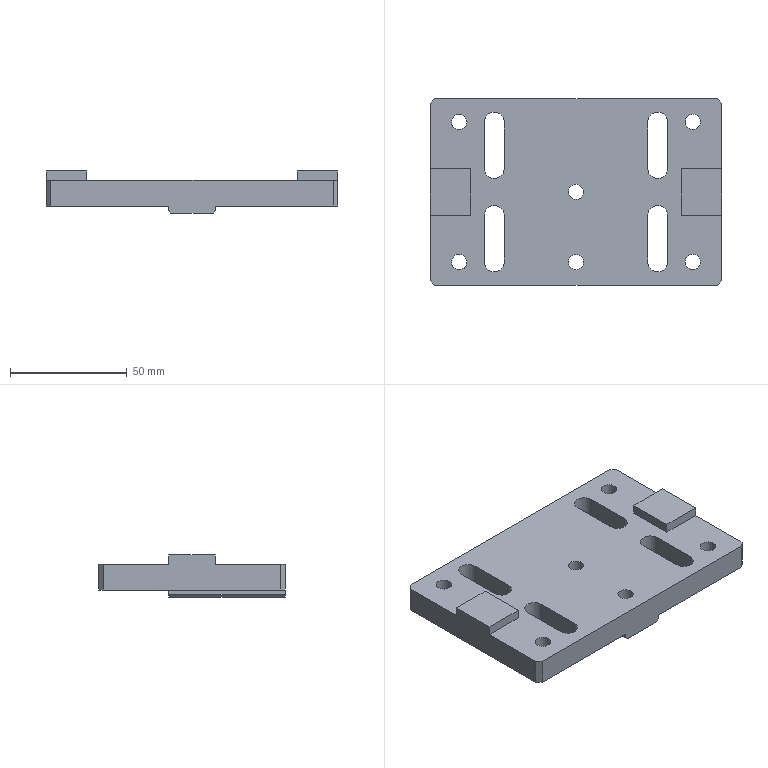NC program | NX | posted with a generic post | part box 125 x 80 x 18 mm
Lines 1 to 631 of 3483:
N10 G17 G21 G94 G90
(FLOOR_WALL , TOOL : D63)
N12 T01 M6
N14 G54
N16 G17 G0 G90 X97. Y-39.997 S6500 M3
N18 G43 Z30. H1
N20 Z3.
N22 G94 G1 Z0. F1500.
N24 X94.
N26 X-94.
N28 Y-32.029
N30 Y-12.599
N32 X94.
N34 Y14.8
N36 X-94.
N38 X-97.
N40 Z3.
N42 G0 Z30.
N44 M5
(FLOOR_WALL_1 , TOOL : D10)
N46 T04 M6
N48 G54
N50 G17 G0 G90 X69. Y1. S7000 M3
N52 G43 Z30. H4
N54 Z0.533
N56 G94 G1 Z-0.967 F1000.
N58 X63.5
N60 G3 X62.5 Y0. R1.
N62 G1 Y-38. F3000.
N64 X60.5 Y-40.
N66 X-60.5
N68 X-62.5 Y-38.
N70 Y38.
N72 X-60.5 Y40.
N74 X-15.1
N76 Y-15.1
N78 X15.1
N80 Y40.
N82 X60.5
N84 X62.5 Y38.
N86 Y0.
N88 X55.5
N90 Y-33.
N92 X-55.5
N94 Y33.
N96 X-22.1
N98 Y-15.1
N100 G3 X-19.493 Y-20.55 R7.
N102 G1 X-23.886 Y-26.
N104 X-48.5
N106 Y26.
N108 X-29.1
N110 Y-15.1
N112 G3 X-23.886 Y-26. R14.
N114 G1 X-35.735 Y-19.
N116 X-41.5
N118 Y19.
N120 X-36.1
N122 Y-15.1
N124 G3 X-35.735 Y-19. R21.
N126 G1 X-23.886 Y-26.
N128 X-19.493 Y-20.55
N130 G3 X-15.1 Y-22.1 R7.
N132 G1 X15.1
N134 G3 X22.1 Y-15.099 R7.
N136 G1 Y33.
N138 X55.5
N140 Y0.
N142 X48.5
N144 Y-26.
N146 X23.886
N148 X18.909 Y-26.479
N150 G2 X15.1 Y-27.1 R12.
N152 G1 X-15.1
N154 G2 X-18.909 Y-26.479 R12.
N156 X-19.303 Y-28. R5.
N158 G1 X19.303
N160 G2 X18.909 Y-26.479 R5.
N162 G1 X23.886 Y-26.
N164 G3 X29.1 Y-15.099 R14.
N166 G1 Y26.
N168 X48.5
N170 Y0.
N172 X41.5
N174 Y-19.
N176 X35.735
N178 G3 X36.1 Y-15.098 R21.
N180 G1 Y19.
N182 X41.5
N184 Y0.
N186 G3 X42.5 Y-1. R1.
N188 G1 Z0.533
N190 G0 X69. Y1. Z-0.433
N192 G1 Z-1.933 F1000.
N194 X63.5
N196 G3 X62.5 Y0. R1.
N198 G1 Y-38. F3000.
N200 X60.5 Y-40.
N202 X-60.5
N204 X-62.5 Y-38.
N206 Y38.
N208 X-60.5 Y40.
N210 X-15.1
N212 Y-15.1
N214 X15.1
N216 Y40.
N218 X60.5
N220 X62.5 Y38.
N222 Y0.
N224 X55.5
N226 Y-33.
N228 X-55.5
N230 Y33.
N232 X-22.1
N234 Y-15.1
N236 G3 X-19.493 Y-20.55 R7.
N238 G1 X-23.886 Y-26.
N240 X-48.5
N242 Y26.
N244 X-29.1
N246 Y-15.1
N248 G3 X-23.886 Y-26. R14.
N250 G1 X-35.735 Y-19.
N252 X-41.5
N254 Y19.
N256 X-36.1
N258 Y-15.1
N260 G3 X-35.735 Y-19. R21.
N262 G1 X-23.886 Y-26.
N264 X-19.493 Y-20.55
N266 G3 X-15.1 Y-22.1 R7.
N268 G1 X15.1
N270 G3 X22.1 Y-15.099 R7.
N272 G1 Y33.
N274 X55.5
N276 Y0.
N278 X48.5
N280 Y-26.
N282 X23.886
N284 X18.909 Y-26.479
N286 G2 X15.1 Y-27.1 R12.
N288 G1 X-15.1
N290 G2 X-18.909 Y-26.479 R12.
N292 X-19.303 Y-28. R5.
N294 G1 X19.303
N296 G2 X18.909 Y-26.479 R5.
N298 G1 X23.886 Y-26.
N300 G3 X29.1 Y-15.099 R14.
N302 G1 Y26.
N304 X48.5
N306 Y0.
N308 X41.5
N310 Y-19.
N312 X35.735
N314 G3 X36.1 Y-15.098 R21.
N316 G1 Y19.
N318 X41.5
N320 Y0.
N322 G3 X42.5 Y-1. R1.
N324 G1 Z-0.433
N326 G0 X69. Y1. Z-1.4
N328 G1 Z-2.9 F1000.
N330 X63.5
N332 G3 X62.5 Y0. R1.
N334 G1 Y-38. F3000.
N336 X60.5 Y-40.
N338 X-60.5
N340 X-62.5 Y-38.
N342 Y38.
N344 X-60.5 Y40.
N346 X-15.1
N348 Y-15.1
N350 X15.1
N352 Y40.
N354 X60.5
N356 X62.5 Y38.
N358 Y0.
N360 X55.5
N362 Y-33.
N364 X-55.5
N366 Y33.
N368 X-22.1
N370 Y-15.1
N372 G3 X-19.493 Y-20.55 R7.
N374 G1 X-23.886 Y-26.
N376 X-48.5
N378 Y26.
N380 X-29.1
N382 Y-15.1
N384 G3 X-23.886 Y-26. R14.
N386 G1 X-35.735 Y-19.
N388 X-41.5
N390 Y19.
N392 X-36.1
N394 Y-15.1
N396 G3 X-35.735 Y-19. R21.
N398 G1 X-23.886 Y-26.
N400 X-19.493 Y-20.55
N402 G3 X-15.1 Y-22.1 R7.
N404 G1 X15.1
N406 G3 X22.1 Y-15.099 R7.
N408 G1 Y33.
N410 X55.5
N412 Y0.
N414 X48.5
N416 Y-26.
N418 X23.886
N420 X18.909 Y-26.479
N422 G2 X15.1 Y-27.1 R12.
N424 G1 X-15.1
N426 G2 X-18.909 Y-26.479 R12.
N428 X-19.303 Y-28. R5.
N430 G1 X19.303
N432 G2 X18.909 Y-26.479 R5.
N434 G1 X23.886 Y-26.
N436 G3 X29.1 Y-15.099 R14.
N438 G1 Y26.
N440 X48.5
N442 Y0.
N444 X41.5
N446 Y-19.
N448 X35.735
N450 G3 X36.1 Y-15.098 R21.
N452 G1 Y19.
N454 X41.5
N456 Y0.
N458 G3 X42.5 Y-1. R1.
N460 G1 Z-1.4
N462 G0 Z30.
(FLOOR_WALL_1_COPY , TOOL : D10)
N464 X63.692 Y46.
N466 Z-1.5
N468 G1 Z-3. F1000.
N470 X63.497
N472 G3 X62.497 Y45. R1.
N474 G1 Y-45. F1200.
N476 X57.657
N478 Y45.
N480 X52.817
N482 Y-45.
N484 X47.977
N486 Y45.
N488 X43.137
N490 Y-45.
N492 X38.298
N494 Y45.
N496 X33.458
N498 Y-45.
N500 X28.618
N502 Y45.
N504 X23.778
N506 Y-45.
N508 X18.938
N510 Y45.
N512 X15.5
N514 Y-15.
N516 G2 X15. Y-15.5 R0.5
N518 G1 X14.098
N520 Y-45.
N522 X9.258
N524 Y-15.5
N526 X4.418
N528 Y-45.
N530 X-0.421
N532 Y-15.5
N534 X-5.261
N536 Y-45.
N538 X-10.101
N540 Y-15.5
N542 X-14.941
N544 Y-45.
N546 X-19.781
N548 Y45.
N550 X-24.621
N552 Y-45.
N554 X-29.461
N556 Y45.
N558 X-34.301
N560 Y-45.
N562 X-39.14
N564 Y45.
N566 X-43.98
N568 Y-45.
N570 X-48.82
N572 Y45.
N574 X-53.66
N576 Y-45.
N578 X-58.5
N580 Y45.
N582 G2 X-57.5 Y46. R1.
N584 G1 Y46.5
N586 Z-1.5
N588 G0 Z1.
N590 G1 X16. F8000.
N592 G0 Z-1.5
N594 G1 Z-3. F1000.
N596 Y46.
N598 G3 X15. Y45. R1.
N600 G1 Y-15. F1200.
N602 X-15.
N604 Y45.
N606 G3 X-16. Y46. R1.
N608 G1 Y46.5
N610 Z-1.5
N612 G0 Z30.
(ZLEVEL_PROFILE_COPY , TOOL : D10)
N614 X64.168 Y45.962
N616 Z-4.
N618 G1 X63.777 Y44.501 F1000.
N620 G3 X64.036 Y43.536 R1.
N622 G1 X66.036 Y41.536 F2000.
N624 G3 X67.001 Y41.277 R1.
N626 G1 X68.462 Y41.668
N628 G0 Z-5.
N630 G1 X67.001 Y41.277 F1000.
N632 G2 X66.036 Y41.536 R1.
N634 G1 X64.036 Y43.536 F2000.
N636 G2 X63.777 Y44.501 R1.
N638 G1 X64.168 Y45.962
N640 G0 Z-6.
N642 G1 X63.777 Y44.501 F1000.
N644 G3 X64.036 Y43.536 R1.
N646 G1 X66.036 Y41.536 F2000.
N648 G3 X67.001 Y41.277 R1.
N650 G1 X68.462 Y41.668
N652 G0 Z-7.
N654 G1 X67.001 Y41.277 F1000.
N656 G2 X66.036 Y41.536 R1.
N658 G1 X64.036 Y43.536 F2000.
N660 G2 X63.777 Y44.501 R1.
N662 G1 X64.168 Y45.962
N664 G0 Z-8.
N666 G1 X63.777 Y44.501 F1000.
N668 G3 X64.036 Y43.536 R1.
N670 G1 X66.036 Y41.536 F2000.
N672 G3 X67.001 Y41.277 R1.
N674 G1 X68.462 Y41.668
N676 G0 Z-9.
N678 G1 X67.001 Y41.277 F1000.
N680 G2 X66.036 Y41.536 R1.
N682 G1 X64.036 Y43.536 F2000.
N684 G2 X63.777 Y44.501 R1.
N686 G1 X64.168 Y45.962
N688 G0 Z-10.
N690 G1 X63.777 Y44.501 F1000.
N692 G3 X64.036 Y43.536 R1.
N694 G1 X66.036 Y41.536 F2000.
N696 G3 X67.001 Y41.277 R1.
N698 G1 X68.462 Y41.668
N700 G0 Z-11.
N702 G1 X67.001 Y41.277 F1000.
N704 G2 X66.036 Y41.536 R1.
N706 G1 X64.036 Y43.536 F2000.
N708 G2 X63.777 Y44.501 R1.
N710 G1 X64.168 Y45.962
N712 G0 Z-12.
N714 G1 X63.777 Y44.501 F1000.
N716 G3 X64.036 Y43.536 R1.
N718 G1 X66.036 Y41.536 F2000.
N720 G3 X67.001 Y41.277 R1.
N722 G1 X68.462 Y41.668
N724 G0 Z-13.
N726 G1 X67.001 Y41.277 F1000.
N728 G2 X66.036 Y41.536 R1.
N730 G1 X64.036 Y43.536 F2000.
N732 G2 X63.777 Y44.501 R1.
N734 G1 X64.168 Y45.962
N736 G0 Z-14.
N738 G1 X63.777 Y44.501 F1000.
N740 G3 X64.036 Y43.536 R1.
N742 G1 X66.036 Y41.536 F2000.
N744 G3 X67.001 Y41.277 R1.
N746 G1 X68.462 Y41.668
N748 G0 Z30.
N750 Y-41.668
N752 Z-4.
N754 G1 X67.001 Y-41.277 F1000.
N756 G3 X66.036 Y-41.536 R1.
N758 G1 X64.036 Y-43.536 F2000.
N760 G3 X63.777 Y-44.501 R1.
N762 G1 X64.168 Y-45.962
N764 G0 Z-5.
N766 G1 X63.777 Y-44.501 F1000.
N768 G2 X64.036 Y-43.536 R1.
N770 G1 X66.036 Y-41.536 F2000.
N772 G2 X67.001 Y-41.277 R1.
N774 G1 X68.462 Y-41.668
N776 G0 Z-6.
N778 G1 X67.001 Y-41.277 F1000.
N780 G3 X66.036 Y-41.536 R1.
N782 G1 X64.036 Y-43.536 F2000.
N784 G3 X63.777 Y-44.501 R1.
N786 G1 X64.168 Y-45.962
N788 G0 Z-7.
N790 G1 X63.777 Y-44.501 F1000.
N792 G2 X64.036 Y-43.536 R1.
N794 G1 X66.036 Y-41.536 F2000.
N796 G2 X67.001 Y-41.277 R1.
N798 G1 X68.462 Y-41.668
N800 G0 Z-8.
N802 G1 X67.001 Y-41.277 F1000.
N804 G3 X66.036 Y-41.536 R1.
N806 G1 X64.036 Y-43.536 F2000.
N808 G3 X63.777 Y-44.501 R1.
N810 G1 X64.168 Y-45.962
N812 G0 Z-9.
N814 G1 X63.777 Y-44.501 F1000.
N816 G2 X64.036 Y-43.536 R1.
N818 G1 X66.036 Y-41.536 F2000.
N820 G2 X67.001 Y-41.277 R1.
N822 G1 X68.462 Y-41.668
N824 G0 Z-10.
N826 G1 X67.001 Y-41.277 F1000.
N828 G3 X66.036 Y-41.536 R1.
N830 G1 X64.036 Y-43.536 F2000.
N832 G3 X63.777 Y-44.501 R1.
N834 G1 X64.168 Y-45.962
N836 G0 Z-11.
N838 G1 X63.777 Y-44.501 F1000.
N840 G2 X64.036 Y-43.536 R1.
N842 G1 X66.036 Y-41.536 F2000.
N844 G2 X67.001 Y-41.277 R1.
N846 G1 X68.462 Y-41.668
N848 G0 Z-12.
N850 G1 X67.001 Y-41.277 F1000.
N852 G3 X66.036 Y-41.536 R1.
N854 G1 X64.036 Y-43.536 F2000.
N856 G3 X63.777 Y-44.501 R1.
N858 G1 X64.168 Y-45.962
N860 G0 Z-13.
N862 G1 X63.777 Y-44.501 F1000.
N864 G2 X64.036 Y-43.536 R1.
N866 G1 X66.036 Y-41.536 F2000.
N868 G2 X67.001 Y-41.277 R1.
N870 G1 X68.462 Y-41.668
N872 G0 Z-14.
N874 G1 X67.001 Y-41.277 F1000.
N876 G3 X66.036 Y-41.536 R1.
N878 G1 X64.036 Y-43.536 F2000.
N880 G3 X63.777 Y-44.501 R1.
N882 G1 X64.168 Y-45.962
N884 G0 Z30.
N886 X-64.168
N888 Z-4.
N890 G1 X-63.777 Y-44.501 F1000.
N892 G3 X-64.036 Y-43.536 R1.
N894 G1 X-66.036 Y-41.536 F2000.
N896 G3 X-67.001 Y-41.277 R1.
N898 G1 X-68.462 Y-41.668
N900 G0 Z-5.
N902 G1 X-67.001 Y-41.277 F1000.
N904 G2 X-66.036 Y-41.536 R1.
N906 G1 X-64.036 Y-43.536 F2000.
N908 G2 X-63.777 Y-44.501 R1.
N910 G1 X-64.168 Y-45.962
N912 G0 Z-6.
N914 G1 X-63.777 Y-44.501 F1000.
N916 G3 X-64.036 Y-43.536 R1.
N918 G1 X-66.036 Y-41.536 F2000.
N920 G3 X-67.001 Y-41.277 R1.
N922 G1 X-68.462 Y-41.668
N924 G0 Z-7.
N926 G1 X-67.001 Y-41.277 F1000.
N928 G2 X-66.036 Y-41.536 R1.
N930 G1 X-64.036 Y-43.536 F2000.
N932 G2 X-63.777 Y-44.501 R1.
N934 G1 X-64.168 Y-45.962
N936 G0 Z-8.
N938 G1 X-63.777 Y-44.501 F1000.
N940 G3 X-64.036 Y-43.536 R1.
N942 G1 X-66.036 Y-41.536 F2000.
N944 G3 X-67.001 Y-41.277 R1.
N946 G1 X-68.462 Y-41.668
N948 G0 Z-9.
N950 G1 X-67.001 Y-41.277 F1000.
N952 G2 X-66.036 Y-41.536 R1.
N954 G1 X-64.036 Y-43.536 F2000.
N956 G2 X-63.777 Y-44.501 R1.
N958 G1 X-64.168 Y-45.962
N960 G0 Z-10.
N962 G1 X-63.777 Y-44.501 F1000.
N964 G3 X-64.036 Y-43.536 R1.
N966 G1 X-66.036 Y-41.536 F2000.
N968 G3 X-67.001 Y-41.277 R1.
N970 G1 X-68.462 Y-41.668
N972 G0 Z-11.
N974 G1 X-67.001 Y-41.277 F1000.
N976 G2 X-66.036 Y-41.536 R1.
N978 G1 X-64.036 Y-43.536 F2000.
N980 G2 X-63.777 Y-44.501 R1.
N982 G1 X-64.168 Y-45.962
N984 G0 Z-12.
N986 G1 X-63.777 Y-44.501 F1000.
N988 G3 X-64.036 Y-43.536 R1.
N990 G1 X-66.036 Y-41.536 F2000.
N992 G3 X-67.001 Y-41.277 R1.
N994 G1 X-68.462 Y-41.668
N996 G0 Z-13.
N998 G1 X-67.001 Y-41.277 F1000.
N1000 G2 X-66.036 Y-41.536 R1.
N1002 G1 X-64.036 Y-43.536 F2000.
N1004 G2 X-63.777 Y-44.501 R1.
N1006 G1 X-64.168 Y-45.962
N1008 G0 Z-14.
N1010 G1 X-63.777 Y-44.501 F1000.
N1012 G3 X-64.036 Y-43.536 R1.
N1014 G1 X-66.036 Y-41.536 F2000.
N1016 G3 X-67.001 Y-41.277 R1.
N1018 G1 X-68.462 Y-41.668
N1020 G0 Z30.
N1022 Y41.668
N1024 Z-4.
N1026 G1 X-67.001 Y41.277 F1000.
N1028 G3 X-66.036 Y41.536 R1.
N1030 G1 X-64.036 Y43.536 F2000.
N1032 G3 X-63.777 Y44.501 R1.
N1034 G1 X-64.168 Y45.962
N1036 G0 Z-5.
N1038 G1 X-63.777 Y44.501 F1000.
N1040 G2 X-64.036 Y43.536 R1.
N1042 G1 X-66.036 Y41.536 F2000.
N1044 G2 X-67.001 Y41.277 R1.
N1046 G1 X-68.462 Y41.668
N1048 G0 Z-6.
N1050 G1 X-67.001 Y41.277 F1000.
N1052 G3 X-66.036 Y41.536 R1.
N1054 G1 X-64.036 Y43.536 F2000.
N1056 G3 X-63.777 Y44.501 R1.
N1058 G1 X-64.168 Y45.962
N1060 G0 Z-7.
N1062 G1 X-63.777 Y44.501 F1000.
N1064 G2 X-64.036 Y43.536 R1.
N1066 G1 X-66.036 Y41.536 F2000.
N1068 G2 X-67.001 Y41.277 R1.
N1070 G1 X-68.462 Y41.668
N1072 G0 Z-8.
N1074 G1 X-67.001 Y41.277 F1000.
N1076 G3 X-66.036 Y41.536 R1.
N1078 G1 X-64.036 Y43.536 F2000.
N1080 G3 X-63.777 Y44.501 R1.
N1082 G1 X-64.168 Y45.962
N1084 G0 Z-9.
N1086 G1 X-63.777 Y44.501 F1000.
N1088 G2 X-64.036 Y43.536 R1.
N1090 G1 X-66.036 Y41.536 F2000.
N1092 G2 X-67.001 Y41.277 R1.
N1094 G1 X-68.462 Y41.668
N1096 G0 Z-10.
N1098 G1 X-67.001 Y41.277 F1000.
N1100 G3 X-66.036 Y41.536 R1.
N1102 G1 X-64.036 Y43.536 F2000.
N1104 G3 X-63.777 Y44.501 R1.
N1106 G1 X-64.168 Y45.962
N1108 G0 Z-11.
N1110 G1 X-63.777 Y44.501 F1000.
N1112 G2 X-64.036 Y43.536 R1.
N1114 G1 X-66.036 Y41.536 F2000.
N1116 G2 X-67.001 Y41.277 R1.
N1118 G1 X-68.462 Y41.668
N1120 G0 Z-12.
N1122 G1 X-67.001 Y41.277 F1000.
N1124 G3 X-66.036 Y41.536 R1.
N1126 G1 X-64.036 Y43.536 F2000.
N1128 G3 X-63.777 Y44.501 R1.
N1130 G1 X-64.168 Y45.962
N1132 G0 Z-13.
N1134 G1 X-63.777 Y44.501 F1000.
N1136 G2 X-64.036 Y43.536 R1.
N1138 G1 X-66.036 Y41.536 F2000.
N1140 G2 X-67.001 Y41.277 R1.
N1142 G1 X-68.462 Y41.668
N1144 G0 Z-14.
N1146 G1 X-67.001 Y41.277 F1000.
N1148 G3 X-66.036 Y41.536 R1.
N1150 G1 X-64.036 Y43.536 F2000.
N1152 G3 X-63.777 Y44.501 R1.
N1154 G1 X-64.168 Y45.962
N1156 G0 Z30.
N1158 M5
(DRILLING , TOOL : D8A45)
N1160 T06 M6
N1162 G54
N1164 G17 G0 G90 X-50. Y-30. S3500 M3
N1166 G43 Z30. H6
N1168 G94 G81 G98 Z-6.35 F250. R0.
N1170 Y30.
N1172 X0. Z-3.35 R3.
N1174 Y0.
N1176 X50. Y-30. Z-6.35 R0.
N1178 Y30.
N1180 G80
N1182 G0 X50. Y30. Z30.
N1184 M5
(DRILLING_2 , TOOL : 6.5ZT)
N1186 T22 M6
N1188 G54
N1190 G17 G0 G90 X0. Y30. S2000 M3
N1192 G43 Z30. H22
N1194 G94 G83 G98 Z-17.453 F250. Q3. R3.
N1196 Y0.
N1198 G80
N1200 G0 X0. Y0. Z30.
N1202 M5
(DRILLING_2_COPY , TOOL : 6.6ZT)
N1204 T23 M6
N1206 G54
N1208 G17 G0 G90 X-50. Y-30. S2000 M3
N1210 G43 Z30. H23
N1212 G94 G83 G98 Z-17.483 F250. Q3. R0.
N1214 Y30.
N1216 X50.
N1218 Y-30.
N1220 G80
N1222 G0 X50. Y-30. Z30.
N1224 M5